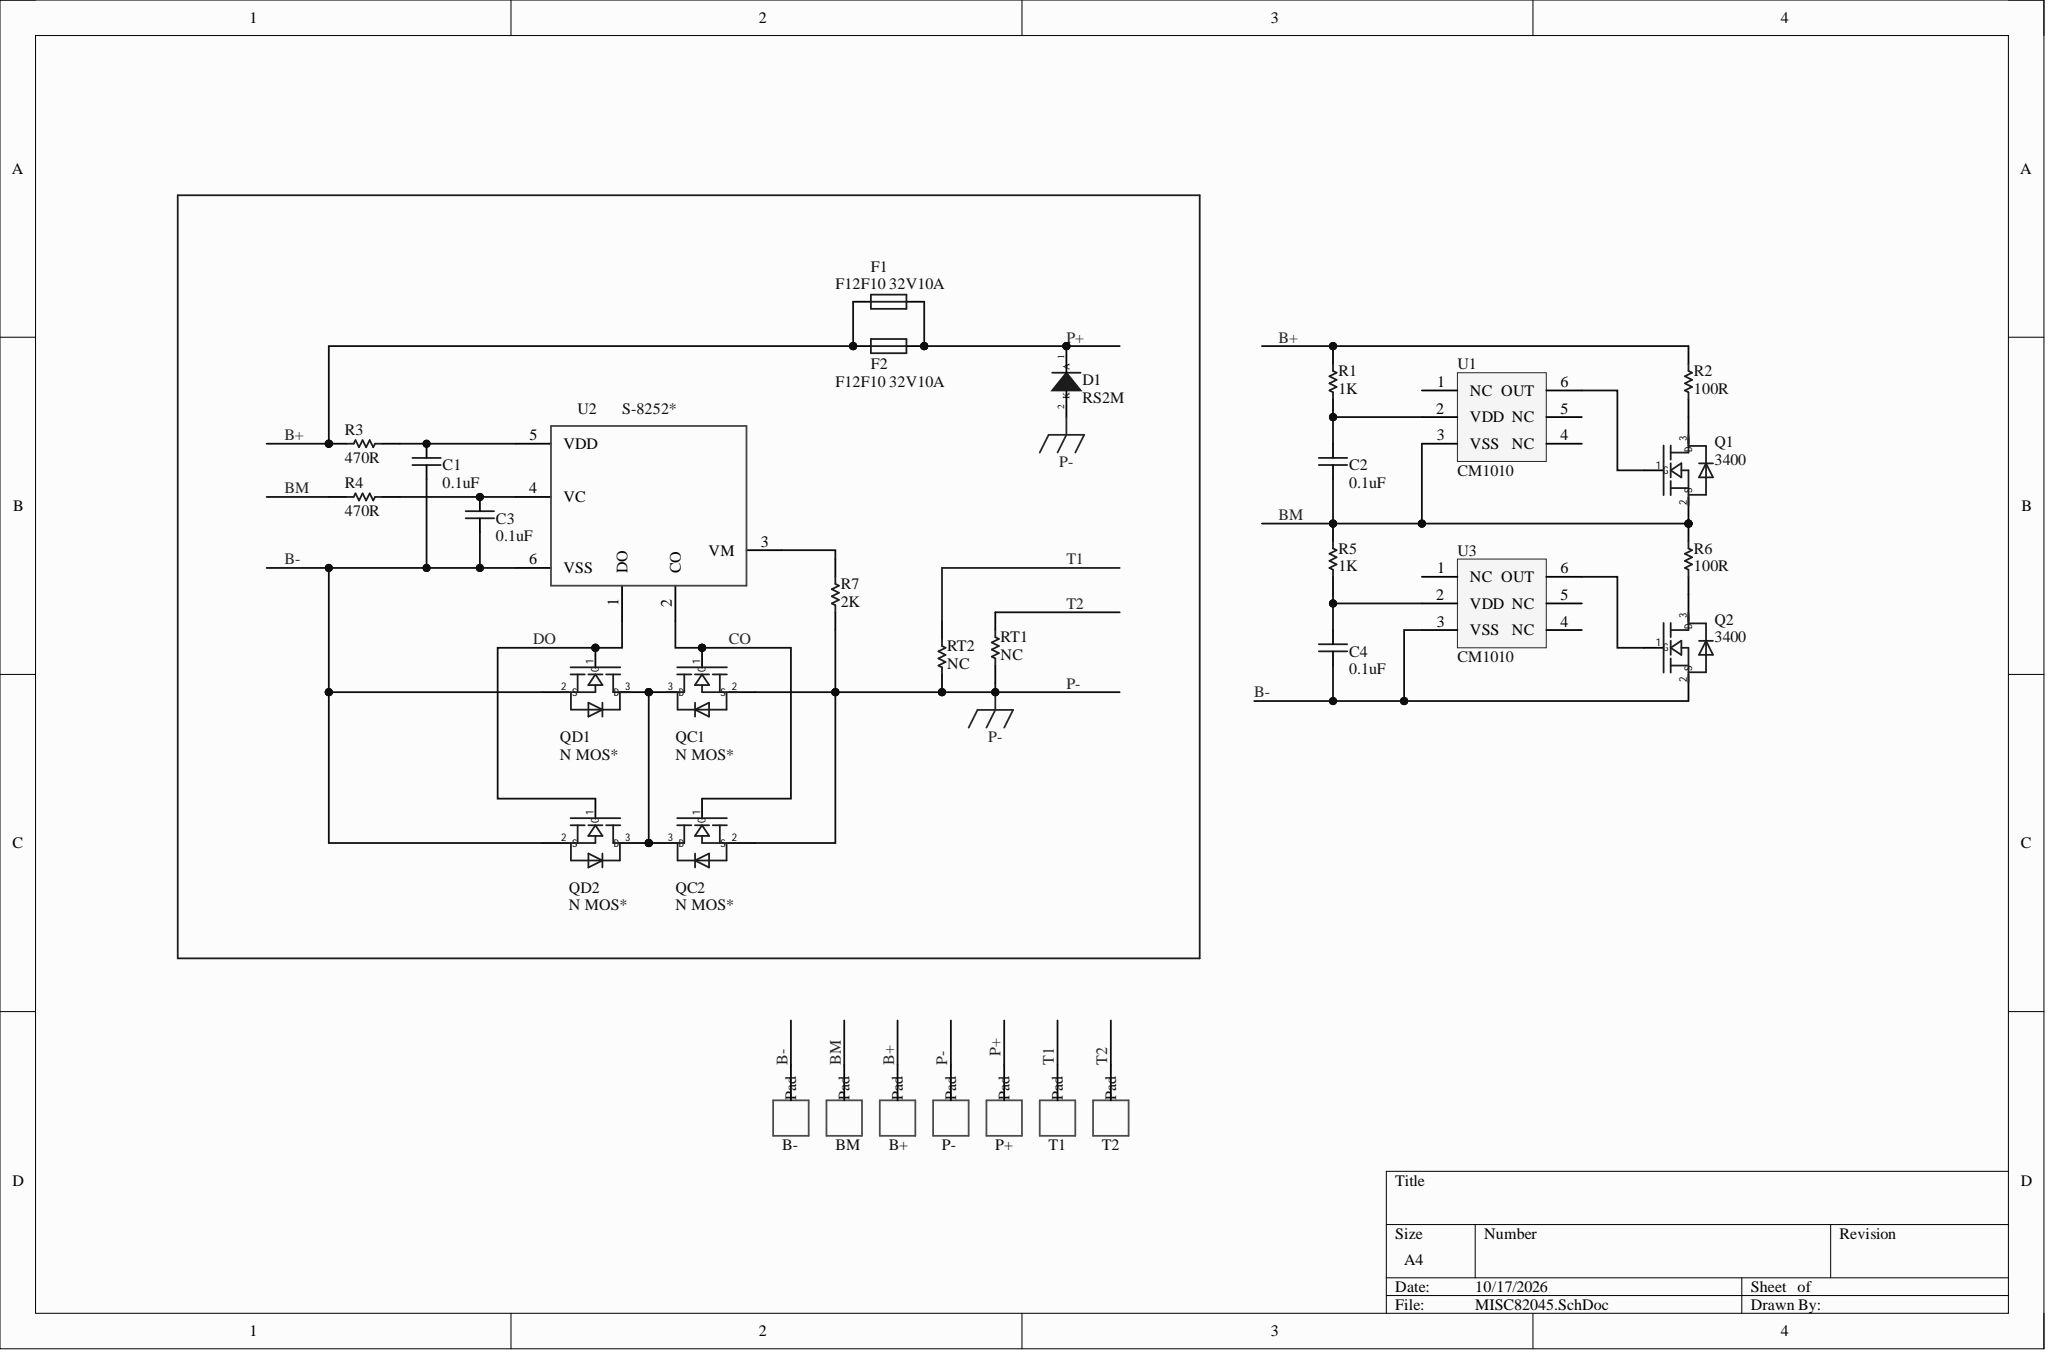Circuit board | Altium Designer | 32 parts | 19 nets
Bill of materials:
Comment,Description,Designator,Footprint,LibRef,Quantity
"Pad","Connection pad (non-through-hole)","B-, B+, BM, P-, P+, T1, T2","Pad10X8mm","Pad","7"
"0.1uF","SMD capacitor","C1, C2, C3, C4","C0603A","CAP","4"
"RS2M","SMD diode","D1","SMB A (1+2-)","RS2M","1"
"F12F10 32V10A","","F1, F2","R1206A","FUSE","2"
"3400","SMD MOSFET","Q1, Q2","SOT23-3L","N MOS*","2"
"N MOS*","SMD MOSFET","QC1, QC2, QD1, QD2","TO-252","N MOS*","4"
"1K","SMD resistor","R1, R5","R0603A","RES","2"
"100R","SMD resistor","R2, R6","R1206A","RES","2"
"470R","SMD resistor","R3, R4","R0603A","RES","2"
"2K","SMD resistor","R7","R0603A","RES","1"
"NC","SMD resistor","RT1, RT2","R0603A","RES","2"
"CM1010","Chuangxinwei, balancing IC","U1, U3","SOT23-6A","CM1010","2"
"S-8252*","2S battery protection IC","U2","SOT23-6A","S-8252","1"
Netlist (Protel format):
[
B+
Pad10X8mm
Pad



]
[
B-
Pad10X8mm
Pad



]
[
BM
Pad10X8mm
Pad



]
[
C1
C0603A
0.1uF



]
[
C2
C0603A
0.1uF



]
[
C3
C0603A
0.1uF



]
[
C4
C0603A
0.1uF



]
[
D1
SMB A (1+2-)
RS2M



]
[
F1
R1206A
F12F10 32V10A



]
[
F2
R1206A
F12F10 32V10A



]
[
P+
Pad10X8mm
Pad



]
[
P-
Pad10X8mm
Pad



]
[
Q1
SOT23-3L
3400



]
[
Q2
SOT23-3L
3400



]
[
QC1
TO-252
N MOS*



]
[
QC2
TO-252
N MOS*



]
[
QD1
TO-252
N MOS*



]
[
QD2
TO-252
N MOS*



]
[
R1
R0603A
1K



]
[
R2
R1206A
100R



]
[
R3
R0603A
470R



]
[
R4
R0603A
470R



]
[
R5
R0603A
1K



]
[
R6
R1206A
100R



]
[
R7
R0603A
2K



]
[
RT1
R0603A
NC



]
[
RT2
R0603A
NC



]
[
T1
Pad10X8mm
Pad



]
[
T2
Pad10X8mm
Pad



]
[
U1
SOT23-6A
CM1010



]
[
U2
SOT23-6A
S-8252*



]
[
U3
SOT23-6A
CM1010



]
(
T2
RT1-2
T2-1
)
(
T1
RT2-2
T1-1
)
(
P-
D1-2
P--1
QC1-2
QC2-2
R7-1
RT1-1
RT2-1
)
(
P+
D1-1
F1-2
F2-2
P+-1
)
(
NetR7_2
R7-2
U2-3
)
(
NetQC1_3
QC1-3
QC2-3
QD1-3
QD2-3
)
(
NetQ2_3
Q2-3
R6-1
)
(
NetQ2_1
Q2-1
U3-6
)
(
NetQ1_3
Q1-3
R2-1
)
(
NetQ1_1
Q1-1
U1-6
)
(
NetC4_2
C4-2
R5-1
U3-2
)
(
NetC3_2
C3-2
R4-2
U2-4
)
(
NetC2_2
C2-2
R1-1
U1-2
)
(
NetC1_2
C1-2
R3-2
U2-5
)
(
DO
QD1-1
QD2-1
U2-1
)
(
CO
QC1-1
QC2-1
U2-2
)
(
BM
BM-1
C2-1
Q1-2
R4-1
R5-2
R6-2
U1-3
)
(
B-
B--1
C1-1
C3-1
C4-1
Q2-2
QD1-2
QD2-2
U2-6
U3-3
)
(
B+
B+-1
F1-1
F2-1
R1-2
R2-2
R3-1
)